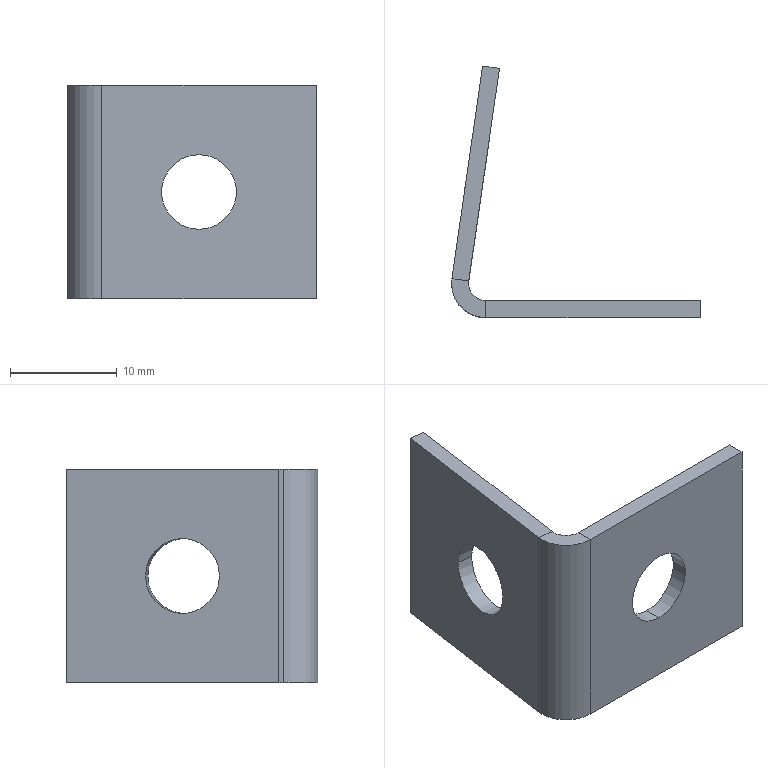Part | SolidWorks | features ICE 2, FlatPattern 1, SMBaseFlange 1, SheetMetal 1 | 1 solid | 20 faces | box 23.305 x 23.556 x 20 mm | volume 1295 mm3 | plane 12 | cylinder 8 | commonest cylinder face diameters 7 x4 3.2 x2 6.4 x2
STEP:
#1=CARTESIAN_POINT('',(3.912,15.904,0.));
#2=VERTEX_POINT('',#1);
#3=CARTESIAN_POINT('',(2.912,8.976,0.));
#4=VERTEX_POINT('',#3);
#5=CARTESIAN_POINT('',(3.412,12.44,0.));
#6=DIRECTION('',(-0.9897,0.1429,0.));
#7=DIRECTION('',(-0.1429,-0.9897,0.));
#8=AXIS2_PLACEMENT_3D('',#5,#6,#7);
#9=CIRCLE('',#8,3.5);
#10=EDGE_CURVE('',#2,#4,#9,.T.);
#11=ORIENTED_EDGE('',*,*,#10,.F.);
#12=CARTESIAN_POINT('',(2.329,16.133,0.));
#13=VERTEX_POINT('',#12);
#14=CARTESIAN_POINT('',(12.226,14.704,0.));
#15=DIRECTION('',(-0.9897,0.1429,0.));
#16=VECTOR('',#15,1000.);
#17=LINE('',#14,#16);
#18=EDGE_CURVE('',#2,#13,#17,.T.);
#19=ORIENTED_EDGE('',*,*,#18,.T.);
#20=CARTESIAN_POINT('',(1.329,9.205,0.));
#21=VERTEX_POINT('',#20);
#22=CARTESIAN_POINT('',(1.829,12.669,0.));
#23=DIRECTION('',(-0.9897,0.1429,0.));
#24=DIRECTION('',(-0.1429,-0.9897,0.));
#25=AXIS2_PLACEMENT_3D('',#22,#23,#24);
#26=CIRCLE('',#25,3.5);
#27=EDGE_CURVE('',#13,#21,#26,.T.);
#28=ORIENTED_EDGE('',*,*,#27,.T.);
#29=CARTESIAN_POINT('',(11.226,7.776,0.));
#30=DIRECTION('',(-0.9897,0.1429,0.));
#31=VECTOR('',#30,1000.);
#32=LINE('',#29,#31);
#33=EDGE_CURVE('',#4,#21,#32,.T.);
#34=ORIENTED_EDGE('',*,*,#33,.F.);
#35=EDGE_LOOP('',(#11,#19,#28,#34));
#36=FACE_OUTER_BOUND('',#35,.T.);
#37=CARTESIAN_POINT('',(11.726,11.24,0.));
#38=DIRECTION('',(-0.9897,0.1429,0.));
#39=DIRECTION('',(-0.1429,-0.9897,0.));
#40=AXIS2_PLACEMENT_3D('',#37,#38,#39);
#41=CYLINDRICAL_SURFACE('',#40,3.5);
#42=ADVANCED_FACE('',(#36),#41,.F.);
#43=CARTESIAN_POINT('',(12.8,1.6,3.5));
#44=VERTEX_POINT('',#43);
#45=CARTESIAN_POINT('',(12.8,1.6,-3.5));
#46=VERTEX_POINT('',#45);
#47=CARTESIAN_POINT('',(12.8,1.6,0.));
#48=DIRECTION('',(0.,-1.,0.));
#49=DIRECTION('',(0.,0.,-1.));
#50=AXIS2_PLACEMENT_3D('',#47,#48,#49);
#51=CIRCLE('',#50,3.5);
#52=EDGE_CURVE('',#44,#46,#51,.T.);
#53=ORIENTED_EDGE('',*,*,#52,.F.);
#54=CARTESIAN_POINT('',(12.8,0.,3.5));
#55=VERTEX_POINT('',#54);
#56=CARTESIAN_POINT('',(12.8,10.,3.5));
#57=DIRECTION('',(0.,-1.,0.));
#58=VECTOR('',#57,1000.);
#59=LINE('',#56,#58);
#60=EDGE_CURVE('',#44,#55,#59,.T.);
#61=ORIENTED_EDGE('',*,*,#60,.T.);
#62=CARTESIAN_POINT('',(12.8,0.,-3.5));
#63=VERTEX_POINT('',#62);
#64=CARTESIAN_POINT('',(12.8,0.,0.));
#65=DIRECTION('',(0.,-1.,0.));
#66=DIRECTION('',(0.,0.,-1.));
#67=AXIS2_PLACEMENT_3D('',#64,#65,#66);
#68=CIRCLE('',#67,3.5);
#69=EDGE_CURVE('',#55,#63,#68,.T.);
#70=ORIENTED_EDGE('',*,*,#69,.T.);
#71=CARTESIAN_POINT('',(12.8,10.,-3.5));
#72=DIRECTION('',(0.,-1.,0.));
#73=VECTOR('',#72,1000.);
#74=LINE('',#71,#73);
#75=EDGE_CURVE('',#46,#63,#74,.T.);
#76=ORIENTED_EDGE('',*,*,#75,.F.);
#77=EDGE_LOOP('',(#53,#61,#70,#76));
#78=FACE_OUTER_BOUND('',#77,.T.);
#79=CARTESIAN_POINT('',(12.8,10.,0.));
#80=DIRECTION('',(0.,-1.,0.));
#81=DIRECTION('',(0.,0.,-1.));
#82=AXIS2_PLACEMENT_3D('',#79,#80,#81);
#83=CYLINDRICAL_SURFACE('',#82,3.5);
#84=ADVANCED_FACE('',(#78),#83,.F.);
#85=CARTESIAN_POINT('',(2.095,3.2,10.));
#86=VERTEX_POINT('',#85);
#87=CARTESIAN_POINT('',(2.111,3.429,10.));
#88=VERTEX_POINT('',#87);
#89=CARTESIAN_POINT('',(3.695,3.2,10.));
#90=DIRECTION('',(0.,0.,-1.));
#91=DIRECTION('',(1.,0.,0.));
#92=AXIS2_PLACEMENT_3D('',#89,#90,#91);
#93=CIRCLE('',#92,1.6);
#94=EDGE_CURVE('',#86,#88,#93,.T.);
#95=ORIENTED_EDGE('',*,*,#94,.F.);
#96=CARTESIAN_POINT('',(2.095,3.2,-10.));
#97=VERTEX_POINT('',#96);
#98=CARTESIAN_POINT('',(2.095,3.2,10.));
#99=DIRECTION('',(0.,0.,-1.));
#100=VECTOR('',#99,1000.);
#101=LINE('',#98,#100);
#102=EDGE_CURVE('',#86,#97,#101,.T.);
#103=ORIENTED_EDGE('',*,*,#102,.T.);
#104=CARTESIAN_POINT('',(2.111,3.429,-10.));
#105=VERTEX_POINT('',#104);
#106=CARTESIAN_POINT('',(3.695,3.2,-10.));
#107=DIRECTION('',(0.,0.,-1.));
#108=DIRECTION('',(1.,0.,0.));
#109=AXIS2_PLACEMENT_3D('',#106,#107,#108);
#110=CIRCLE('',#109,1.6);
#111=EDGE_CURVE('',#97,#105,#110,.T.);
#112=ORIENTED_EDGE('',*,*,#111,.T.);
#113=CARTESIAN_POINT('',(2.111,3.429,10.));
#114=DIRECTION('',(0.,0.,-1.));
#115=VECTOR('',#114,1000.);
#116=LINE('',#113,#115);
#117=EDGE_CURVE('',#88,#105,#116,.T.);
#118=ORIENTED_EDGE('',*,*,#117,.F.);
#119=EDGE_LOOP('',(#95,#103,#112,#118));
#120=FACE_OUTER_BOUND('',#119,.T.);
#121=CARTESIAN_POINT('',(3.695,3.2,10.));
#122=DIRECTION('',(0.,0.,-1.));
#123=DIRECTION('',(-1.,0.,0.));
#124=AXIS2_PLACEMENT_3D('',#121,#122,#123);
#125=CYLINDRICAL_SURFACE('',#124,1.6);
#126=ADVANCED_FACE('',(#120),#125,.F.);
#127=CARTESIAN_POINT('',(3.695,0.,10.));
#128=VERTEX_POINT('',#127);
#129=CARTESIAN_POINT('',(0.495,3.2,10.));
#130=VERTEX_POINT('',#129);
#131=CARTESIAN_POINT('',(3.695,3.2,10.));
#132=DIRECTION('',(0.,0.,-1.));
#133=DIRECTION('',(1.,0.,0.));
#134=AXIS2_PLACEMENT_3D('',#131,#132,#133);
#135=CIRCLE('',#134,3.2);
#136=EDGE_CURVE('',#128,#130,#135,.T.);
#137=ORIENTED_EDGE('',*,*,#136,.T.);
#138=CARTESIAN_POINT('',(0.495,3.2,-10.));
#139=VERTEX_POINT('',#138);
#140=CARTESIAN_POINT('',(0.495,3.2,10.));
#141=DIRECTION('',(0.,0.,-1.));
#142=VECTOR('',#141,1000.);
#143=LINE('',#140,#142);
#144=EDGE_CURVE('',#130,#139,#143,.T.);
#145=ORIENTED_EDGE('',*,*,#144,.T.);
#146=CARTESIAN_POINT('',(3.695,0.,-10.));
#147=VERTEX_POINT('',#146);
#148=CARTESIAN_POINT('',(3.695,3.2,-10.));
#149=DIRECTION('',(0.,0.,-1.));
#150=DIRECTION('',(1.,0.,0.));
#151=AXIS2_PLACEMENT_3D('',#148,#149,#150);
#152=CIRCLE('',#151,3.2);
#153=EDGE_CURVE('',#147,#139,#152,.T.);
#154=ORIENTED_EDGE('',*,*,#153,.F.);
#155=CARTESIAN_POINT('',(3.695,0.,10.));
#156=DIRECTION('',(0.,0.,-1.));
#157=VECTOR('',#156,1000.);
#158=LINE('',#155,#157);
#159=EDGE_CURVE('',#128,#147,#158,.T.);
#160=ORIENTED_EDGE('',*,*,#159,.F.);
#161=EDGE_LOOP('',(#137,#145,#154,#160));
#162=FACE_OUTER_BOUND('',#161,.T.);
#163=CARTESIAN_POINT('',(3.695,3.2,10.));
#164=DIRECTION('',(0.,0.,-1.));
#165=DIRECTION('',(-1.,0.,0.));
#166=AXIS2_PLACEMENT_3D('',#163,#164,#165);
#167=CYLINDRICAL_SURFACE('',#166,3.2);
#168=ADVANCED_FACE('',(#162),#167,.T.);
#169=CARTESIAN_POINT('',(0.5279,3.657,10.));
#170=VERTEX_POINT('',#169);
#171=CARTESIAN_POINT('',(0.5279,3.657,10.));
#172=DIRECTION('',(0.9897,-0.1429,0.));
#173=VECTOR('',#172,1000.);
#174=LINE('',#171,#173);
#175=EDGE_CURVE('',#170,#88,#174,.T.);
#176=ORIENTED_EDGE('',*,*,#175,.F.);
#177=CARTESIAN_POINT('',(3.695,3.2,10.));
#178=DIRECTION('',(0.,0.,-1.));
#179=DIRECTION('',(1.,0.,0.));
#180=AXIS2_PLACEMENT_3D('',#177,#178,#179);
#181=CIRCLE('',#180,3.2);
#182=EDGE_CURVE('',#130,#170,#181,.T.);
#183=ORIENTED_EDGE('',*,*,#182,.F.);
#184=ORIENTED_EDGE('',*,*,#136,.F.);
#185=CARTESIAN_POINT('',(3.695,1.6,10.));
#186=VERTEX_POINT('',#185);
#187=CARTESIAN_POINT('',(3.695,1.6,10.));
#188=DIRECTION('',(0.,-1.,0.));
#189=VECTOR('',#188,1000.);
#190=LINE('',#187,#189);
#191=EDGE_CURVE('',#186,#128,#190,.T.);
#192=ORIENTED_EDGE('',*,*,#191,.F.);
#193=CARTESIAN_POINT('',(3.695,3.2,10.));
#194=DIRECTION('',(0.,0.,-1.));
#195=DIRECTION('',(1.,0.,0.));
#196=AXIS2_PLACEMENT_3D('',#193,#194,#195);
#197=CIRCLE('',#196,1.6);
#198=EDGE_CURVE('',#186,#86,#197,.T.);
#199=ORIENTED_EDGE('',*,*,#198,.T.);
#200=ORIENTED_EDGE('',*,*,#94,.T.);
#201=EDGE_LOOP('',(#176,#183,#184,#192,#199,#200));
#202=FACE_OUTER_BOUND('',#201,.T.);
#203=CARTESIAN_POINT('',(0.5279,3.657,10.));
#204=DIRECTION('',(0.,0.,1.));
#205=DIRECTION('',(1.,0.,0.));
#206=AXIS2_PLACEMENT_3D('',#203,#204,#205);
#207=PLANE('',#206);
#208=ADVANCED_FACE('',(#202),#207,.T.);
#209=CARTESIAN_POINT('',(3.4,23.556,10.));
#210=VERTEX_POINT('',#209);
#211=CARTESIAN_POINT('',(0.,0.,10.));
#212=DIRECTION('',(0.1429,0.9897,0.));
#213=VECTOR('',#212,1000.);
#214=LINE('',#211,#213);
#215=EDGE_CURVE('',#170,#210,#214,.T.);
#216=ORIENTED_EDGE('',*,*,#215,.F.);
#217=ORIENTED_EDGE('',*,*,#175,.T.);
#218=CARTESIAN_POINT('',(4.984,23.327,10.));
#219=VERTEX_POINT('',#218);
#220=CARTESIAN_POINT('',(1.584,-0.2286,10.));
#221=DIRECTION('',(0.1429,0.9897,0.));
#222=VECTOR('',#221,1000.);
#223=LINE('',#220,#222);
#224=EDGE_CURVE('',#88,#219,#223,.T.);
#225=ORIENTED_EDGE('',*,*,#224,.T.);
#226=CARTESIAN_POINT('',(3.4,23.556,10.));
#227=DIRECTION('',(0.9897,-0.1429,0.));
#228=VECTOR('',#227,1000.);
#229=LINE('',#226,#228);
#230=EDGE_CURVE('',#210,#219,#229,.T.);
#231=ORIENTED_EDGE('',*,*,#230,.F.);
#232=EDGE_LOOP('',(#216,#217,#225,#231));
#233=FACE_OUTER_BOUND('',#232,.T.);
#234=CARTESIAN_POINT('',(3.695,1.6,10.));
#235=DIRECTION('',(0.,0.,1.));
#236=DIRECTION('',(1.,0.,0.));
#237=AXIS2_PLACEMENT_3D('',#234,#235,#236);
#238=PLANE('',#237);
#239=ADVANCED_FACE('',(#233),#238,.T.);
#240=CARTESIAN_POINT('',(3.695,1.6,-10.));
#241=VERTEX_POINT('',#240);
#242=CARTESIAN_POINT('',(3.695,0.,-10.));
#243=DIRECTION('',(0.,1.,0.));
#244=VECTOR('',#243,1000.);
#245=LINE('',#242,#244);
#246=EDGE_CURVE('',#147,#241,#245,.T.);
#247=ORIENTED_EDGE('',*,*,#246,.F.);
#248=ORIENTED_EDGE('',*,*,#153,.T.);
#249=CARTESIAN_POINT('',(0.5279,3.657,-10.));
#250=VERTEX_POINT('',#249);
#251=CARTESIAN_POINT('',(3.695,3.2,-10.));
#252=DIRECTION('',(0.,0.,-1.));
#253=DIRECTION('',(1.,0.,0.));
#254=AXIS2_PLACEMENT_3D('',#251,#252,#253);
#255=CIRCLE('',#254,3.2);
#256=EDGE_CURVE('',#139,#250,#255,.T.);
#257=ORIENTED_EDGE('',*,*,#256,.T.);
#258=CARTESIAN_POINT('',(2.111,3.429,-10.));
#259=DIRECTION('',(-0.9897,0.1429,0.));
#260=VECTOR('',#259,1000.);
#261=LINE('',#258,#260);
#262=EDGE_CURVE('',#105,#250,#261,.T.);
#263=ORIENTED_EDGE('',*,*,#262,.F.);
#264=ORIENTED_EDGE('',*,*,#111,.F.);
#265=CARTESIAN_POINT('',(3.695,3.2,-10.));
#266=DIRECTION('',(0.,0.,-1.));
#267=DIRECTION('',(1.,0.,0.));
#268=AXIS2_PLACEMENT_3D('',#265,#266,#267);
#269=CIRCLE('',#268,1.6);
#270=EDGE_CURVE('',#241,#97,#269,.T.);
#271=ORIENTED_EDGE('',*,*,#270,.F.);
#272=EDGE_LOOP('',(#247,#248,#257,#263,#264,#271));
#273=FACE_OUTER_BOUND('',#272,.T.);
#274=CARTESIAN_POINT('',(3.695,0.,-10.));
#275=DIRECTION('',(0.,0.,-1.));
#276=DIRECTION('',(-1.,0.,0.));
#277=AXIS2_PLACEMENT_3D('',#274,#275,#276);
#278=PLANE('',#277);
#279=ADVANCED_FACE('',(#273),#278,.T.);
#280=CARTESIAN_POINT('',(23.8,0.,-10.));
#281=VERTEX_POINT('',#280);
#282=CARTESIAN_POINT('',(23.8,0.,-10.));
#283=DIRECTION('',(-1.,0.,0.));
#284=VECTOR('',#283,1000.);
#285=LINE('',#282,#284);
#286=EDGE_CURVE('',#281,#147,#285,.T.);
#287=ORIENTED_EDGE('',*,*,#286,.T.);
#288=ORIENTED_EDGE('',*,*,#246,.T.);
#289=CARTESIAN_POINT('',(23.8,1.6,-10.));
#290=VERTEX_POINT('',#289);
#291=CARTESIAN_POINT('',(23.8,1.6,-10.));
#292=DIRECTION('',(-1.,0.,0.));
#293=VECTOR('',#292,1000.);
#294=LINE('',#291,#293);
#295=EDGE_CURVE('',#290,#241,#294,.T.);
#296=ORIENTED_EDGE('',*,*,#295,.F.);
#297=CARTESIAN_POINT('',(23.8,1.6,-10.));
#298=DIRECTION('',(0.,-1.,0.));
#299=VECTOR('',#298,1000.);
#300=LINE('',#297,#299);
#301=EDGE_CURVE('',#290,#281,#300,.T.);
#302=ORIENTED_EDGE('',*,*,#301,.T.);
#303=EDGE_LOOP('',(#287,#288,#296,#302));
#304=FACE_OUTER_BOUND('',#303,.T.);
#305=CARTESIAN_POINT('',(2.111,3.429,-10.));
#306=DIRECTION('',(0.,0.,-1.));
#307=DIRECTION('',(-1.,0.,0.));
#308=AXIS2_PLACEMENT_3D('',#305,#306,#307);
#309=PLANE('',#308);
#310=ADVANCED_FACE('',(#304),#309,.T.);
#311=CARTESIAN_POINT('',(3.412,12.44,0.));
#312=DIRECTION('',(-0.9897,0.1429,0.));
#313=DIRECTION('',(-0.1429,-0.9897,0.));
#314=AXIS2_PLACEMENT_3D('',#311,#312,#313);
#315=CIRCLE('',#314,3.5);
#316=EDGE_CURVE('',#4,#2,#315,.T.);
#317=ORIENTED_EDGE('',*,*,#316,.T.);
#318=ORIENTED_EDGE('',*,*,#10,.T.);
#319=EDGE_LOOP('',(#317,#318));
#320=FACE_BOUND('',#319,.T.);
#321=CARTESIAN_POINT('',(4.984,23.327,-10.));
#322=VERTEX_POINT('',#321);
#323=CARTESIAN_POINT('',(1.584,-0.2286,-10.));
#324=DIRECTION('',(0.1429,0.9897,0.));
#325=VECTOR('',#324,1000.);
#326=LINE('',#323,#325);
#327=EDGE_CURVE('',#105,#322,#326,.T.);
#328=ORIENTED_EDGE('',*,*,#327,.T.);
#329=CARTESIAN_POINT('',(4.984,23.327,10.));
#330=DIRECTION('',(0.,0.,-1.));
#331=VECTOR('',#330,1000.);
#332=LINE('',#329,#331);
#333=EDGE_CURVE('',#219,#322,#332,.T.);
#334=ORIENTED_EDGE('',*,*,#333,.F.);
#335=ORIENTED_EDGE('',*,*,#224,.F.);
#336=ORIENTED_EDGE('',*,*,#117,.T.);
#337=EDGE_LOOP('',(#328,#334,#335,#336));
#338=FACE_OUTER_BOUND('',#337,.T.);
#339=CARTESIAN_POINT('',(1.584,-0.2286,10.));
#340=DIRECTION('',(-0.9897,0.1429,0.));
#341=DIRECTION('',(-0.1429,-0.9897,0.));
#342=AXIS2_PLACEMENT_3D('',#339,#340,#341);
#343=PLANE('',#342);
#344=ADVANCED_FACE('',(#320,#338),#343,.F.);
#345=CARTESIAN_POINT('',(3.4,23.556,-10.));
#346=VERTEX_POINT('',#345);
#347=CARTESIAN_POINT('',(3.4,23.556,-10.));
#348=DIRECTION('',(0.9897,-0.1429,0.));
#349=VECTOR('',#348,1000.);
#350=LINE('',#347,#349);
#351=EDGE_CURVE('',#346,#322,#350,.T.);
#352=ORIENTED_EDGE('',*,*,#351,.F.);
#353=CARTESIAN_POINT('',(3.4,23.556,10.));
#354=DIRECTION('',(0.,0.,-1.));
#355=VECTOR('',#354,1000.);
#356=LINE('',#353,#355);
#357=EDGE_CURVE('',#210,#346,#356,.T.);
#358=ORIENTED_EDGE('',*,*,#357,.F.);
#359=ORIENTED_EDGE('',*,*,#230,.T.);
#360=ORIENTED_EDGE('',*,*,#333,.T.);
#361=EDGE_LOOP('',(#352,#358,#359,#360));
#362=FACE_OUTER_BOUND('',#361,.T.);
#363=CARTESIAN_POINT('',(3.4,23.556,10.));
#364=DIRECTION('',(0.1429,0.9897,0.));
#365=DIRECTION('',(-0.9897,0.1429,0.));
#366=AXIS2_PLACEMENT_3D('',#363,#364,#365);
#367=PLANE('',#366);
#368=ADVANCED_FACE('',(#362),#367,.T.);
#369=CARTESIAN_POINT('',(1.829,12.669,0.));
#370=DIRECTION('',(-0.9897,0.1429,0.));
#371=DIRECTION('',(-0.1429,-0.9897,0.));
#372=AXIS2_PLACEMENT_3D('',#369,#370,#371);
#373=CIRCLE('',#372,3.5);
#374=EDGE_CURVE('',#21,#13,#373,.T.);
#375=ORIENTED_EDGE('',*,*,#374,.F.);
#376=ORIENTED_EDGE('',*,*,#27,.F.);
#377=EDGE_LOOP('',(#375,#376));
#378=FACE_BOUND('',#377,.T.);
#379=CARTESIAN_POINT('',(0.,0.,-10.));
#380=DIRECTION('',(0.1429,0.9897,0.));
#381=VECTOR('',#380,1000.);
#382=LINE('',#379,#381);
#383=EDGE_CURVE('',#250,#346,#382,.T.);
#384=ORIENTED_EDGE('',*,*,#383,.F.);
#385=CARTESIAN_POINT('',(0.5279,3.657,10.));
#386=DIRECTION('',(0.,0.,-1.));
#387=VECTOR('',#386,1000.);
#388=LINE('',#385,#387);
#389=EDGE_CURVE('',#170,#250,#388,.T.);
#390=ORIENTED_EDGE('',*,*,#389,.F.);
#391=ORIENTED_EDGE('',*,*,#215,.T.);
#392=ORIENTED_EDGE('',*,*,#357,.T.);
#393=EDGE_LOOP('',(#384,#390,#391,#392));
#394=FACE_OUTER_BOUND('',#393,.T.);
#395=CARTESIAN_POINT('',(0.,0.,10.));
#396=DIRECTION('',(-0.9897,0.1429,0.));
#397=DIRECTION('',(-0.1429,-0.9897,0.));
#398=AXIS2_PLACEMENT_3D('',#395,#396,#397);
#399=PLANE('',#398);
#400=ADVANCED_FACE('',(#378,#394),#399,.T.);
#401=ORIENTED_EDGE('',*,*,#144,.F.);
#402=ORIENTED_EDGE('',*,*,#182,.T.);
#403=ORIENTED_EDGE('',*,*,#389,.T.);
#404=ORIENTED_EDGE('',*,*,#256,.F.);
#405=EDGE_LOOP('',(#401,#402,#403,#404));
#406=FACE_OUTER_BOUND('',#405,.T.);
#407=CARTESIAN_POINT('',(3.695,3.2,10.));
#408=DIRECTION('',(0.,0.,-1.));
#409=DIRECTION('',(-1.,0.,0.));
#410=AXIS2_PLACEMENT_3D('',#407,#408,#409);
#411=CYLINDRICAL_SURFACE('',#410,3.2);
#412=ADVANCED_FACE('',(#406),#411,.T.);
#413=CARTESIAN_POINT('',(12.8,0.,0.));
#414=DIRECTION('',(0.,-1.,0.));
#415=DIRECTION('',(0.,0.,-1.));
#416=AXIS2_PLACEMENT_3D('',#413,#414,#415);
#417=CIRCLE('',#416,3.5);
#418=EDGE_CURVE('',#63,#55,#417,.T.);
#419=ORIENTED_EDGE('',*,*,#418,.F.);
#420=ORIENTED_EDGE('',*,*,#69,.F.);
#421=EDGE_LOOP('',(#419,#420));
#422=FACE_BOUND('',#421,.T.);
#423=ORIENTED_EDGE('',*,*,#286,.F.);
#424=CARTESIAN_POINT('',(23.8,0.,10.));
#425=VERTEX_POINT('',#424);
#426=CARTESIAN_POINT('',(23.8,0.,10.));
#427=DIRECTION('',(0.,0.,-1.));
#428=VECTOR('',#427,1000.);
#429=LINE('',#426,#428);
#430=EDGE_CURVE('',#425,#281,#429,.T.);
#431=ORIENTED_EDGE('',*,*,#430,.F.);
#432=CARTESIAN_POINT('',(23.8,0.,10.));
#433=DIRECTION('',(-1.,0.,0.));
#434=VECTOR('',#433,1000.);
#435=LINE('',#432,#434);
#436=EDGE_CURVE('',#425,#128,#435,.T.);
#437=ORIENTED_EDGE('',*,*,#436,.T.);
#438=ORIENTED_EDGE('',*,*,#159,.T.);
#439=EDGE_LOOP('',(#423,#431,#437,#438));
#440=FACE_OUTER_BOUND('',#439,.T.);
#441=CARTESIAN_POINT('',(23.8,0.,10.));
#442=DIRECTION('',(0.,-1.,0.));
#443=DIRECTION('',(0.,0.,-1.));
#444=AXIS2_PLACEMENT_3D('',#441,#442,#443);
#445=PLANE('',#444);
#446=ADVANCED_FACE('',(#422,#440),#445,.T.);
#447=ORIENTED_EDGE('',*,*,#301,.F.);
#448=CARTESIAN_POINT('',(23.8,1.6,10.));
#449=VERTEX_POINT('',#448);
#450=CARTESIAN_POINT('',(23.8,1.6,10.));
#451=DIRECTION('',(0.,0.,-1.));
#452=VECTOR('',#451,1000.);
#453=LINE('',#450,#452);
#454=EDGE_CURVE('',#449,#290,#453,.T.);
#455=ORIENTED_EDGE('',*,*,#454,.F.);
#456=CARTESIAN_POINT('',(23.8,1.6,10.));
#457=DIRECTION('',(0.,-1.,0.));
#458=VECTOR('',#457,1000.);
#459=LINE('',#456,#458);
#460=EDGE_CURVE('',#449,#425,#459,.T.);
#461=ORIENTED_EDGE('',*,*,#460,.T.);
#462=ORIENTED_EDGE('',*,*,#430,.T.);
#463=EDGE_LOOP('',(#447,#455,#461,#462));
#464=FACE_OUTER_BOUND('',#463,.T.);
#465=CARTESIAN_POINT('',(23.8,1.6,10.));
#466=DIRECTION('',(1.,0.,0.));
#467=DIRECTION('',(0.,0.,-1.));
#468=AXIS2_PLACEMENT_3D('',#465,#466,#467);
#469=PLANE('',#468);
#470=ADVANCED_FACE('',(#464),#469,.T.);
#471=CARTESIAN_POINT('',(12.8,1.6,0.));
#472=DIRECTION('',(0.,-1.,0.));
#473=DIRECTION('',(0.,0.,-1.));
#474=AXIS2_PLACEMENT_3D('',#471,#472,#473);
#475=CIRCLE('',#474,3.5);
#476=EDGE_CURVE('',#46,#44,#475,.T.);
#477=ORIENTED_EDGE('',*,*,#476,.T.);
#478=ORIENTED_EDGE('',*,*,#52,.T.);
#479=EDGE_LOOP('',(#477,#478));
#480=FACE_BOUND('',#479,.T.);
#481=ORIENTED_EDGE('',*,*,#295,.T.);
#482=CARTESIAN_POINT('',(3.695,1.6,10.));
#483=DIRECTION('',(0.,0.,-1.));
#484=VECTOR('',#483,1000.);
#485=LINE('',#482,#484);
#486=EDGE_CURVE('',#186,#241,#485,.T.);
#487=ORIENTED_EDGE('',*,*,#486,.F.);
#488=CARTESIAN_POINT('',(23.8,1.6,10.));
#489=DIRECTION('',(-1.,0.,0.));
#490=VECTOR('',#489,1000.);
#491=LINE('',#488,#490);
#492=EDGE_CURVE('',#449,#186,#491,.T.);
#493=ORIENTED_EDGE('',*,*,#492,.F.);
#494=ORIENTED_EDGE('',*,*,#454,.T.);
#495=EDGE_LOOP('',(#481,#487,#493,#494));
#496=FACE_OUTER_BOUND('',#495,.T.);
#497=CARTESIAN_POINT('',(23.8,1.6,10.));
#498=DIRECTION('',(0.,-1.,0.));
#499=DIRECTION('',(0.,0.,-1.));
#500=AXIS2_PLACEMENT_3D('',#497,#498,#499);
#501=PLANE('',#500);
#502=ADVANCED_FACE('',(#480,#496),#501,.F.);
#503=ORIENTED_EDGE('',*,*,#102,.F.);
#504=ORIENTED_EDGE('',*,*,#198,.F.);
#505=ORIENTED_EDGE('',*,*,#486,.T.);
#506=ORIENTED_EDGE('',*,*,#270,.T.);
#507=EDGE_LOOP('',(#503,#504,#505,#506));
#508=FACE_OUTER_BOUND('',#507,.T.);
#509=CARTESIAN_POINT('',(3.695,3.2,10.));
#510=DIRECTION('',(0.,0.,-1.));
#511=DIRECTION('',(-1.,0.,0.));
#512=AXIS2_PLACEMENT_3D('',#509,#510,#511);
#513=CYLINDRICAL_SURFACE('',#512,1.6);
#514=ADVANCED_FACE('',(#508),#513,.F.);
#515=ORIENTED_EDGE('',*,*,#492,.T.);
#516=ORIENTED_EDGE('',*,*,#191,.T.);
#517=ORIENTED_EDGE('',*,*,#436,.F.);
#518=ORIENTED_EDGE('',*,*,#460,.F.);
#519=EDGE_LOOP('',(#515,#516,#517,#518));
#520=FACE_OUTER_BOUND('',#519,.T.);
#521=CARTESIAN_POINT('',(3.695,3.2,10.));
#522=DIRECTION('',(0.,0.,1.));
#523=DIRECTION('',(1.,0.,0.));
#524=AXIS2_PLACEMENT_3D('',#521,#522,#523);
#525=PLANE('',#524);
#526=ADVANCED_FACE('',(#520),#525,.T.);
#527=ORIENTED_EDGE('',*,*,#327,.F.);
#528=ORIENTED_EDGE('',*,*,#262,.T.);
#529=ORIENTED_EDGE('',*,*,#383,.T.);
#530=ORIENTED_EDGE('',*,*,#351,.T.);
#531=EDGE_LOOP('',(#527,#528,#529,#530));
#532=FACE_OUTER_BOUND('',#531,.T.);
#533=CARTESIAN_POINT('',(3.695,3.2,-10.));
#534=DIRECTION('',(0.,0.,1.));
#535=DIRECTION('',(1.,0.,0.));
#536=AXIS2_PLACEMENT_3D('',#533,#534,#535);
#537=PLANE('',#536);
#538=ADVANCED_FACE('',(#532),#537,.F.);
#539=ORIENTED_EDGE('',*,*,#60,.F.);
#540=ORIENTED_EDGE('',*,*,#476,.F.);
#541=ORIENTED_EDGE('',*,*,#75,.T.);
#542=ORIENTED_EDGE('',*,*,#418,.T.);
#543=EDGE_LOOP('',(#539,#540,#541,#542));
#544=FACE_OUTER_BOUND('',#543,.T.);
#545=CARTESIAN_POINT('',(12.8,10.,0.));
#546=DIRECTION('',(0.,-1.,0.));
#547=DIRECTION('',(0.,0.,-1.));
#548=AXIS2_PLACEMENT_3D('',#545,#546,#547);
#549=CYLINDRICAL_SURFACE('',#548,3.5);
#550=ADVANCED_FACE('',(#544),#549,.F.);
#551=ORIENTED_EDGE('',*,*,#18,.F.);
#552=ORIENTED_EDGE('',*,*,#316,.F.);
#553=ORIENTED_EDGE('',*,*,#33,.T.);
#554=ORIENTED_EDGE('',*,*,#374,.T.);
#555=EDGE_LOOP('',(#551,#552,#553,#554));
#556=FACE_OUTER_BOUND('',#555,.T.);
#557=CARTESIAN_POINT('',(11.726,11.24,0.));
#558=DIRECTION('',(-0.9897,0.1429,0.));
#559=DIRECTION('',(-0.1429,-0.9897,0.));
#560=AXIS2_PLACEMENT_3D('',#557,#558,#559);
#561=CYLINDRICAL_SURFACE('',#560,3.5);
#562=ADVANCED_FACE('',(#556),#561,.F.);
#563=CLOSED_SHELL('',(#42,#84,#126,#168,#208,#239,#279,#310,#344,#368,#400,#412,#446,#470,#502,#514,#526,#538,#550,#562));
#564=MANIFOLD_SOLID_BREP('',#563);
#565=CARTESIAN_POINT('',(0.,0.,0.));
#566=DIRECTION('',(0.,0.,1.));
#567=DIRECTION('',(1.,0.,0.));
#568=AXIS2_PLACEMENT_3D('',#565,#566,#567);
#569=(LENGTH_UNIT()NAMED_UNIT(*)SI_UNIT(.MILLI.,.METRE.));
#570=UNCERTAINTY_MEASURE_WITH_UNIT(LENGTH_MEASURE(0.00001),#569,'','');
#571=(NAMED_UNIT(*)PLANE_ANGLE_UNIT()SI_UNIT($,.RADIAN.));
#572=(NAMED_UNIT(*)SI_UNIT($,.STERADIAN.)SOLID_ANGLE_UNIT());
#573=(GEOMETRIC_REPRESENTATION_CONTEXT(3)GLOBAL_UNCERTAINTY_ASSIGNED_CONTEXT((#570))GLOBAL_UNIT_ASSIGNED_CONTEXT((#569,#571,#572))REPRESENTATION_CONTEXT('',''));
#574=ADVANCED_BREP_SHAPE_REPRESENTATION('',(#564,#568),#573);